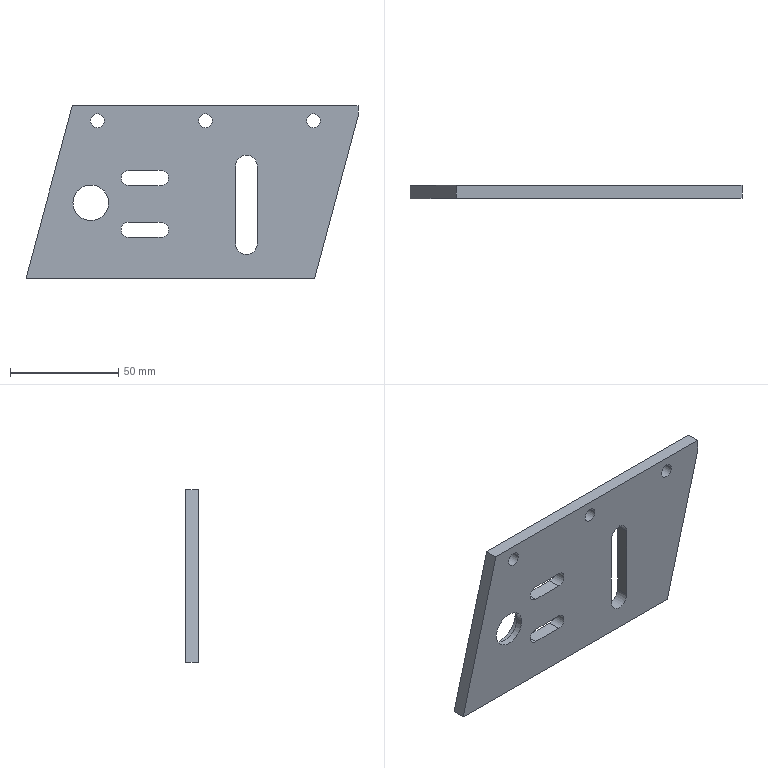Part | SolidWorks | features BaseBody 1 | 1 solid | 32 faces | box 153.66 x 6 x 80 mm | volume 57575 mm3 | cylinder 18 | plane 14 | commonest cylinder face diameters 6.4 x6 7 x6 10 x2 16.5 x2 20 x2
STEP:
#1=CARTESIAN_POINT('',(-37.5,3.,-10.));
#2=VERTEX_POINT('',#1);
#3=CARTESIAN_POINT('',(-37.5,6.,-10.));
#4=VERTEX_POINT('',#3);
#5=CARTESIAN_POINT('',(-37.5,3.,-10.));
#6=DIRECTION('',(0.,1.,0.));
#7=VECTOR('',#6,1000.);
#8=LINE('',#5,#7);
#9=EDGE_CURVE('',#2,#4,#8,.T.);
#10=ORIENTED_EDGE('',*,*,#9,.F.);
#11=CARTESIAN_POINT('',(-57.5,3.,-10.));
#12=VERTEX_POINT('',#11);
#13=CARTESIAN_POINT('',(-47.5,3.,-10.));
#14=DIRECTION('',(0.,1.,0.));
#15=DIRECTION('',(-1.,0.,0.));
#16=AXIS2_PLACEMENT_3D('',#13,#14,#15);
#17=CIRCLE('',#16,10.);
#18=EDGE_CURVE('',#12,#2,#17,.T.);
#19=ORIENTED_EDGE('',*,*,#18,.F.);
#20=CARTESIAN_POINT('',(-57.5,6.,-10.));
#21=VERTEX_POINT('',#20);
#22=CARTESIAN_POINT('',(-57.5,3.,-10.));
#23=DIRECTION('',(0.,1.,0.));
#24=VECTOR('',#23,1000.);
#25=LINE('',#22,#24);
#26=EDGE_CURVE('',#12,#21,#25,.T.);
#27=ORIENTED_EDGE('',*,*,#26,.T.);
#28=CARTESIAN_POINT('',(-47.5,6.,-10.));
#29=DIRECTION('',(0.,-1.,0.));
#30=DIRECTION('',(-1.,0.,0.));
#31=AXIS2_PLACEMENT_3D('',#28,#29,#30);
#32=CIRCLE('',#31,10.);
#33=EDGE_CURVE('',#4,#21,#32,.T.);
#34=ORIENTED_EDGE('',*,*,#33,.F.);
#35=EDGE_LOOP('',(#10,#19,#27,#34));
#36=FACE_OUTER_BOUND('',#35,.T.);
#37=CARTESIAN_POINT('',(-47.5,3.,-10.));
#38=DIRECTION('',(0.,1.,0.));
#39=DIRECTION('',(-1.,0.,0.));
#40=AXIS2_PLACEMENT_3D('',#37,#38,#39);
#41=CYLINDRICAL_SURFACE('',#40,10.);
#42=ADVANCED_FACE('',(#36),#41,.F.);
#43=CARTESIAN_POINT('',(-39.25,3.,-10.));
#44=VERTEX_POINT('',#43);
#45=CARTESIAN_POINT('',(-55.75,3.,-10.));
#46=VERTEX_POINT('',#45);
#47=CARTESIAN_POINT('',(-47.5,3.,-10.));
#48=DIRECTION('',(0.,-1.,0.));
#49=DIRECTION('',(1.,0.,0.));
#50=AXIS2_PLACEMENT_3D('',#47,#48,#49);
#51=CIRCLE('',#50,8.25);
#52=EDGE_CURVE('',#44,#46,#51,.T.);
#53=ORIENTED_EDGE('',*,*,#52,.T.);
#54=CARTESIAN_POINT('',(-47.5,3.,-10.));
#55=DIRECTION('',(0.,-1.,0.));
#56=DIRECTION('',(1.,0.,0.));
#57=AXIS2_PLACEMENT_3D('',#54,#55,#56);
#58=CIRCLE('',#57,8.25);
#59=EDGE_CURVE('',#46,#44,#58,.T.);
#60=ORIENTED_EDGE('',*,*,#59,.T.);
#61=EDGE_LOOP('',(#53,#60));
#62=FACE_BOUND('',#61,.T.);
#63=ORIENTED_EDGE('',*,*,#18,.T.);
#64=CARTESIAN_POINT('',(-47.5,3.,-10.));
#65=DIRECTION('',(0.,1.,0.));
#66=DIRECTION('',(-1.,0.,0.));
#67=AXIS2_PLACEMENT_3D('',#64,#65,#66);
#68=CIRCLE('',#67,10.);
#69=EDGE_CURVE('',#2,#12,#68,.T.);
#70=ORIENTED_EDGE('',*,*,#69,.T.);
#71=EDGE_LOOP('',(#63,#70));
#72=FACE_OUTER_BOUND('',#71,.T.);
#73=CARTESIAN_POINT('',(-47.5,3.,-10.));
#74=DIRECTION('',(0.,1.,0.));
#75=DIRECTION('',(1.,0.,0.));
#76=AXIS2_PLACEMENT_3D('',#73,#74,#75);
#77=PLANE('',#76);
#78=ADVANCED_FACE('',(#62,#72),#77,.T.);
#79=CARTESIAN_POINT('',(-41.3,6.,28.));
#80=VERTEX_POINT('',#79);
#81=CARTESIAN_POINT('',(-47.7,6.,28.));
#82=VERTEX_POINT('',#81);
#83=CARTESIAN_POINT('',(-44.5,6.,28.));
#84=DIRECTION('',(0.,-1.,0.));
#85=DIRECTION('',(1.,0.,0.));
#86=AXIS2_PLACEMENT_3D('',#83,#84,#85);
#87=CIRCLE('',#86,3.2);
#88=EDGE_CURVE('',#80,#82,#87,.T.);
#89=ORIENTED_EDGE('',*,*,#88,.T.);
#90=CARTESIAN_POINT('',(-44.5,6.,28.));
#91=DIRECTION('',(0.,-1.,0.));
#92=DIRECTION('',(1.,0.,0.));
#93=AXIS2_PLACEMENT_3D('',#90,#91,#92);
#94=CIRCLE('',#93,3.2);
#95=EDGE_CURVE('',#82,#80,#94,.T.);
#96=ORIENTED_EDGE('',*,*,#95,.T.);
#97=EDGE_LOOP('',(#89,#96));
#98=FACE_BOUND('',#97,.T.);
#99=CARTESIAN_POINT('',(8.7,6.,28.));
#100=VERTEX_POINT('',#99);
#101=CARTESIAN_POINT('',(2.3,6.,28.));
#102=VERTEX_POINT('',#101);
#103=CARTESIAN_POINT('',(5.5,6.,28.));
#104=DIRECTION('',(0.,-1.,0.));
#105=DIRECTION('',(1.,0.,0.));
#106=AXIS2_PLACEMENT_3D('',#103,#104,#105);
#107=CIRCLE('',#106,3.2);
#108=EDGE_CURVE('',#100,#102,#107,.T.);
#109=ORIENTED_EDGE('',*,*,#108,.T.);
#110=CARTESIAN_POINT('',(5.5,6.,28.));
#111=DIRECTION('',(0.,-1.,0.));
#112=DIRECTION('',(1.,0.,0.));
#113=AXIS2_PLACEMENT_3D('',#110,#111,#112);
#114=CIRCLE('',#113,3.2);
#115=EDGE_CURVE('',#102,#100,#114,.T.);
#116=ORIENTED_EDGE('',*,*,#115,.T.);
#117=EDGE_LOOP('',(#109,#116));
#118=FACE_BOUND('',#117,.T.);
#119=CARTESIAN_POINT('',(58.7,6.,28.));
#120=VERTEX_POINT('',#119);
#121=CARTESIAN_POINT('',(52.3,6.,28.));
#122=VERTEX_POINT('',#121);
#123=CARTESIAN_POINT('',(55.5,6.,28.));
#124=DIRECTION('',(0.,-1.,0.));
#125=DIRECTION('',(1.,0.,0.));
#126=AXIS2_PLACEMENT_3D('',#123,#124,#125);
#127=CIRCLE('',#126,3.2);
#128=EDGE_CURVE('',#120,#122,#127,.T.);
#129=ORIENTED_EDGE('',*,*,#128,.T.);
#130=CARTESIAN_POINT('',(55.5,6.,28.));
#131=DIRECTION('',(0.,-1.,0.));
#132=DIRECTION('',(1.,0.,0.));
#133=AXIS2_PLACEMENT_3D('',#130,#131,#132);
#134=CIRCLE('',#133,3.2);
#135=EDGE_CURVE('',#122,#120,#134,.T.);
#136=ORIENTED_EDGE('',*,*,#135,.T.);
#137=EDGE_LOOP('',(#129,#136));
#138=FACE_BOUND('',#137,.T.);
#139=CARTESIAN_POINT('',(19.5,6.,-29.));
#140=VERTEX_POINT('',#139);
#141=CARTESIAN_POINT('',(29.5,6.,-29.));
#142=VERTEX_POINT('',#141);
#143=CARTESIAN_POINT('',(24.5,6.,-29.));
#144=DIRECTION('',(0.,-1.,0.));
#145=DIRECTION('',(-1.,0.,0.));
#146=AXIS2_PLACEMENT_3D('',#143,#144,#145);
#147=CIRCLE('',#146,5.);
#148=EDGE_CURVE('',#140,#142,#147,.T.);
#149=ORIENTED_EDGE('',*,*,#148,.T.);
#150=CARTESIAN_POINT('',(29.5,6.,7.));
#151=VERTEX_POINT('',#150);
#152=CARTESIAN_POINT('',(29.5,6.,-29.));
#153=DIRECTION('',(0.,0.,1.));
#154=VECTOR('',#153,1000.);
#155=LINE('',#152,#154);
#156=EDGE_CURVE('',#142,#151,#155,.T.);
#157=ORIENTED_EDGE('',*,*,#156,.T.);
#158=CARTESIAN_POINT('',(19.5,6.,7.));
#159=VERTEX_POINT('',#158);
#160=CARTESIAN_POINT('',(24.5,6.,7.));
#161=DIRECTION('',(0.,-1.,0.));
#162=DIRECTION('',(-1.,0.,0.));
#163=AXIS2_PLACEMENT_3D('',#160,#161,#162);
#164=CIRCLE('',#163,5.);
#165=EDGE_CURVE('',#151,#159,#164,.T.);
#166=ORIENTED_EDGE('',*,*,#165,.T.);
#167=CARTESIAN_POINT('',(19.5,6.,-29.));
#168=DIRECTION('',(0.,0.,-1.));
#169=VECTOR('',#168,1000.);
#170=LINE('',#167,#169);
#171=EDGE_CURVE('',#159,#140,#170,.T.);
#172=ORIENTED_EDGE('',*,*,#171,.T.);
#173=EDGE_LOOP('',(#149,#157,#166,#172));
#174=FACE_BOUND('',#173,.T.);
#175=CARTESIAN_POINT('',(-47.5,6.,-10.));
#176=DIRECTION('',(0.,-1.,0.));
#177=DIRECTION('',(-1.,0.,0.));
#178=AXIS2_PLACEMENT_3D('',#175,#176,#177);
#179=CIRCLE('',#178,10.);
#180=EDGE_CURVE('',#21,#4,#179,.T.);
#181=ORIENTED_EDGE('',*,*,#180,.T.);
#182=ORIENTED_EDGE('',*,*,#33,.T.);
#183=EDGE_LOOP('',(#181,#182));
#184=FACE_BOUND('',#183,.T.);
#185=CARTESIAN_POINT('',(-30.,6.,-19.));
#186=VERTEX_POINT('',#185);
#187=CARTESIAN_POINT('',(-33.5,6.,-22.5));
#188=VERTEX_POINT('',#187);
#189=CARTESIAN_POINT('',(-30.,6.,-22.5));
#190=DIRECTION('',(0.,-1.,0.));
#191=DIRECTION('',(-1.,0.,0.));
#192=AXIS2_PLACEMENT_3D('',#189,#190,#191);
#193=CIRCLE('',#192,3.5);
#194=EDGE_CURVE('',#186,#188,#193,.T.);
#195=ORIENTED_EDGE('',*,*,#194,.T.);
#196=CARTESIAN_POINT('',(-30.,6.,-26.));
#197=VERTEX_POINT('',#196);
#198=CARTESIAN_POINT('',(-30.,6.,-22.5));
#199=DIRECTION('',(0.,-1.,0.));
#200=DIRECTION('',(-1.,0.,0.));
#201=AXIS2_PLACEMENT_3D('',#198,#199,#200);
#202=CIRCLE('',#201,3.5);
#203=EDGE_CURVE('',#188,#197,#202,.T.);
#204=ORIENTED_EDGE('',*,*,#203,.T.);
#205=CARTESIAN_POINT('',(-15.,6.,-26.));
#206=VERTEX_POINT('',#205);
#207=CARTESIAN_POINT('',(-30.,6.,-26.));
#208=DIRECTION('',(1.,0.,0.));
#209=VECTOR('',#208,1000.);
#210=LINE('',#207,#209);
#211=EDGE_CURVE('',#197,#206,#210,.T.);
#212=ORIENTED_EDGE('',*,*,#211,.T.);
#213=CARTESIAN_POINT('',(-15.,6.,-19.));
#214=VERTEX_POINT('',#213);
#215=CARTESIAN_POINT('',(-15.,6.,-22.5));
#216=DIRECTION('',(0.,-1.,0.));
#217=DIRECTION('',(-1.,0.,0.));
#218=AXIS2_PLACEMENT_3D('',#215,#216,#217);
#219=CIRCLE('',#218,3.5);
#220=EDGE_CURVE('',#206,#214,#219,.T.);
#221=ORIENTED_EDGE('',*,*,#220,.T.);
#222=CARTESIAN_POINT('',(-30.,6.,-19.));
#223=DIRECTION('',(-1.,0.,0.));
#224=VECTOR('',#223,1000.);
#225=LINE('',#222,#224);
#226=EDGE_CURVE('',#214,#186,#225,.T.);
#227=ORIENTED_EDGE('',*,*,#226,.T.);
#228=EDGE_LOOP('',(#195,#204,#212,#221,#227));
#229=FACE_BOUND('',#228,.T.);
#230=CARTESIAN_POINT('',(-30.,6.,5.));
#231=VERTEX_POINT('',#230);
#232=CARTESIAN_POINT('',(-33.5,6.,1.5));
#233=VERTEX_POINT('',#232);
#234=CARTESIAN_POINT('',(-30.,6.,1.5));
#235=DIRECTION('',(0.,-1.,0.));
#236=DIRECTION('',(-1.,0.,0.));
#237=AXIS2_PLACEMENT_3D('',#234,#235,#236);
#238=CIRCLE('',#237,3.5);
#239=EDGE_CURVE('',#231,#233,#238,.T.);
#240=ORIENTED_EDGE('',*,*,#239,.T.);
#241=CARTESIAN_POINT('',(-30.,6.,-2.));
#242=VERTEX_POINT('',#241);
#243=CARTESIAN_POINT('',(-30.,6.,1.5));
#244=DIRECTION('',(0.,-1.,0.));
#245=DIRECTION('',(-1.,0.,0.));
#246=AXIS2_PLACEMENT_3D('',#243,#244,#245);
#247=CIRCLE('',#246,3.5);
#248=EDGE_CURVE('',#233,#242,#247,.T.);
#249=ORIENTED_EDGE('',*,*,#248,.T.);
#250=CARTESIAN_POINT('',(-15.,6.,-2.));
#251=VERTEX_POINT('',#250);
#252=CARTESIAN_POINT('',(-30.,6.,-2.));
#253=DIRECTION('',(1.,0.,0.));
#254=VECTOR('',#253,1000.);
#255=LINE('',#252,#254);
#256=EDGE_CURVE('',#242,#251,#255,.T.);
#257=ORIENTED_EDGE('',*,*,#256,.T.);
#258=CARTESIAN_POINT('',(-15.,6.,5.));
#259=VERTEX_POINT('',#258);
#260=CARTESIAN_POINT('',(-15.,6.,1.5));
#261=DIRECTION('',(0.,-1.,0.));
#262=DIRECTION('',(-1.,0.,0.));
#263=AXIS2_PLACEMENT_3D('',#260,#261,#262);
#264=CIRCLE('',#263,3.5);
#265=EDGE_CURVE('',#251,#259,#264,.T.);
#266=ORIENTED_EDGE('',*,*,#265,.T.);
#267=CARTESIAN_POINT('',(-30.,6.,5.));
#268=DIRECTION('',(-1.,0.,0.));
#269=VECTOR('',#268,1000.);
#270=LINE('',#267,#269);
#271=EDGE_CURVE('',#259,#231,#270,.T.);
#272=ORIENTED_EDGE('',*,*,#271,.T.);
#273=EDGE_LOOP('',(#240,#249,#257,#266,#272));
#274=FACE_BOUND('',#273,.T.);
#275=CARTESIAN_POINT('',(76.16,6.,30.));
#276=VERTEX_POINT('',#275);
#277=CARTESIAN_POINT('',(56.064,6.,-45.));
#278=VERTEX_POINT('',#277);
#279=CARTESIAN_POINT('',(77.5,6.,35.));
#280=DIRECTION('',(-0.2588,0.,-0.9659));
#281=VECTOR('',#280,1000.);
#282=LINE('',#279,#281);
#283=EDGE_CURVE('',#276,#278,#282,.T.);
#284=ORIENTED_EDGE('',*,*,#283,.T.);
#285=CARTESIAN_POINT('',(-77.5,6.,-45.));
#286=VERTEX_POINT('',#285);
#287=CARTESIAN_POINT('',(-77.5,6.,-45.));
#288=DIRECTION('',(-1.,0.,0.));
#289=VECTOR('',#288,1000.);
#290=LINE('',#287,#289);
#291=EDGE_CURVE('',#278,#286,#290,.T.);
#292=ORIENTED_EDGE('',*,*,#291,.T.);
#293=CARTESIAN_POINT('',(-56.064,6.,35.));
#294=VERTEX_POINT('',#293);
#295=CARTESIAN_POINT('',(-77.5,6.,-45.));
#296=DIRECTION('',(0.2588,0.,0.9659));
#297=VECTOR('',#296,1000.);
#298=LINE('',#295,#297);
#299=EDGE_CURVE('',#286,#294,#298,.T.);
#300=ORIENTED_EDGE('',*,*,#299,.T.);
#301=CARTESIAN_POINT('',(76.16,6.,35.));
#302=VERTEX_POINT('',#301);
#303=CARTESIAN_POINT('',(-77.5,6.,35.));
#304=DIRECTION('',(1.,0.,0.));
#305=VECTOR('',#304,1000.);
#306=LINE('',#303,#305);
#307=EDGE_CURVE('',#294,#302,#306,.T.);
#308=ORIENTED_EDGE('',*,*,#307,.T.);
#309=CARTESIAN_POINT('',(76.16,6.,35.));
#310=DIRECTION('',(0.,0.,-1.));
#311=VECTOR('',#310,1000.);
#312=LINE('',#309,#311);
#313=EDGE_CURVE('',#302,#276,#312,.T.);
#314=ORIENTED_EDGE('',*,*,#313,.T.);
#315=EDGE_LOOP('',(#284,#292,#300,#308,#314));
#316=FACE_OUTER_BOUND('',#315,.T.);
#317=CARTESIAN_POINT('',(0.,6.,0.));
#318=DIRECTION('',(0.,1.,0.));
#319=DIRECTION('',(1.,0.,0.));
#320=AXIS2_PLACEMENT_3D('',#317,#318,#319);
#321=PLANE('',#320);
#322=ADVANCED_FACE('',(#98,#118,#138,#174,#184,#229,#274,#316),#321,.T.);
#323=CARTESIAN_POINT('',(76.16,0.,30.));
#324=VERTEX_POINT('',#323);
#325=CARTESIAN_POINT('',(56.064,0.,-45.));
#326=VERTEX_POINT('',#325);
#327=CARTESIAN_POINT('',(76.16,0.,30.));
#328=DIRECTION('',(-0.2588,0.,-0.9659));
#329=VECTOR('',#328,1000.);
#330=LINE('',#327,#329);
#331=EDGE_CURVE('',#324,#326,#330,.T.);
#332=ORIENTED_EDGE('',*,*,#331,.T.);
#333=CARTESIAN_POINT('',(56.064,6.,-45.));
#334=DIRECTION('',(0.,1.,0.));
#335=VECTOR('',#334,1000.);
#336=LINE('',#333,#335);
#337=EDGE_CURVE('',#326,#278,#336,.T.);
#338=ORIENTED_EDGE('',*,*,#337,.T.);
#339=ORIENTED_EDGE('',*,*,#283,.F.);
#340=CARTESIAN_POINT('',(76.16,6.,30.));
#341=DIRECTION('',(0.,-1.,0.));
#342=VECTOR('',#341,1000.);
#343=LINE('',#340,#342);
#344=EDGE_CURVE('',#276,#324,#343,.T.);
#345=ORIENTED_EDGE('',*,*,#344,.T.);
#346=EDGE_LOOP('',(#332,#338,#339,#345));
#347=FACE_OUTER_BOUND('',#346,.T.);
#348=CARTESIAN_POINT('',(77.5,0.,35.));
#349=DIRECTION('',(-0.9659,0.,0.2588));
#350=DIRECTION('',(0.,1.,0.));
#351=AXIS2_PLACEMENT_3D('',#348,#349,#350);
#352=PLANE('',#351);
#353=ADVANCED_FACE('',(#347),#352,.F.);
#354=CARTESIAN_POINT('',(-77.5,0.,-45.));
#355=VERTEX_POINT('',#354);
#356=CARTESIAN_POINT('',(0.,0.,-45.));
#357=DIRECTION('',(-1.,0.,0.));
#358=VECTOR('',#357,1000.);
#359=LINE('',#356,#358);
#360=EDGE_CURVE('',#326,#355,#359,.T.);
#361=ORIENTED_EDGE('',*,*,#360,.T.);
#362=CARTESIAN_POINT('',(-77.5,0.,-45.));
#363=DIRECTION('',(0.,1.,0.));
#364=VECTOR('',#363,1000.);
#365=LINE('',#362,#364);
#366=EDGE_CURVE('',#355,#286,#365,.T.);
#367=ORIENTED_EDGE('',*,*,#366,.T.);
#368=ORIENTED_EDGE('',*,*,#291,.F.);
#369=ORIENTED_EDGE('',*,*,#337,.F.);
#370=EDGE_LOOP('',(#361,#367,#368,#369));
#371=FACE_OUTER_BOUND('',#370,.T.);
#372=CARTESIAN_POINT('',(-77.5,6.,-45.));
#373=DIRECTION('',(0.,0.,1.));
#374=DIRECTION('',(0.,-1.,0.));
#375=AXIS2_PLACEMENT_3D('',#372,#373,#374);
#376=PLANE('',#375);
#377=ADVANCED_FACE('',(#371),#376,.F.);
#378=ORIENTED_EDGE('',*,*,#299,.F.);
#379=ORIENTED_EDGE('',*,*,#366,.F.);
#380=CARTESIAN_POINT('',(-56.064,0.,35.));
#381=VERTEX_POINT('',#380);
#382=CARTESIAN_POINT('',(-77.5,0.,-45.));
#383=DIRECTION('',(0.2588,0.,0.9659));
#384=VECTOR('',#383,1000.);
#385=LINE('',#382,#384);
#386=EDGE_CURVE('',#355,#381,#385,.T.);
#387=ORIENTED_EDGE('',*,*,#386,.T.);
#388=CARTESIAN_POINT('',(-56.064,6.,35.));
#389=DIRECTION('',(0.,1.,0.));
#390=VECTOR('',#389,1000.);
#391=LINE('',#388,#390);
#392=EDGE_CURVE('',#381,#294,#391,.T.);
#393=ORIENTED_EDGE('',*,*,#392,.T.);
#394=EDGE_LOOP('',(#378,#379,#387,#393));
#395=FACE_OUTER_BOUND('',#394,.T.);
#396=CARTESIAN_POINT('',(-77.5,0.,-45.));
#397=DIRECTION('',(0.9659,0.,-0.2588));
#398=DIRECTION('',(0.,-1.,0.));
#399=AXIS2_PLACEMENT_3D('',#396,#397,#398);
#400=PLANE('',#399);
#401=ADVANCED_FACE('',(#395),#400,.F.);
#402=ORIENTED_EDGE('',*,*,#307,.F.);
#403=ORIENTED_EDGE('',*,*,#392,.F.);
#404=CARTESIAN_POINT('',(76.16,0.,35.));
#405=VERTEX_POINT('',#404);
#406=CARTESIAN_POINT('',(0.,0.,35.));
#407=DIRECTION('',(1.,0.,0.));
#408=VECTOR('',#407,1000.);
#409=LINE('',#406,#408);
#410=EDGE_CURVE('',#381,#405,#409,.T.);
#411=ORIENTED_EDGE('',*,*,#410,.T.);
#412=CARTESIAN_POINT('',(76.16,6.,35.));
#413=DIRECTION('',(0.,1.,0.));
#414=VECTOR('',#413,1000.);
#415=LINE('',#412,#414);
#416=EDGE_CURVE('',#405,#302,#415,.T.);
#417=ORIENTED_EDGE('',*,*,#416,.T.);
#418=EDGE_LOOP('',(#402,#403,#411,#417));
#419=FACE_OUTER_BOUND('',#418,.T.);
#420=CARTESIAN_POINT('',(-77.5,6.,35.));
#421=DIRECTION('',(0.,0.,-1.));
#422=DIRECTION('',(-1.,0.,0.));
#423=AXIS2_PLACEMENT_3D('',#420,#421,#422);
#424=PLANE('',#423);
#425=ADVANCED_FACE('',(#419),#424,.F.);
#426=ORIENTED_EDGE('',*,*,#313,.F.);
#427=ORIENTED_EDGE('',*,*,#416,.F.);
#428=CARTESIAN_POINT('',(76.16,0.,0.));
#429=DIRECTION('',(0.,0.,-1.));
#430=VECTOR('',#429,1000.);
#431=LINE('',#428,#430);
#432=EDGE_CURVE('',#405,#324,#431,.T.);
#433=ORIENTED_EDGE('',*,*,#432,.T.);
#434=ORIENTED_EDGE('',*,*,#344,.F.);
#435=EDGE_LOOP('',(#426,#427,#433,#434));
#436=FACE_OUTER_BOUND('',#435,.T.);
#437=CARTESIAN_POINT('',(76.16,6.,35.));
#438=DIRECTION('',(-1.,0.,0.));
#439=DIRECTION('',(0.,0.,1.));
#440=AXIS2_PLACEMENT_3D('',#437,#438,#439);
#441=PLANE('',#440);
#442=ADVANCED_FACE('',(#436),#441,.F.);
#443=CARTESIAN_POINT('',(-47.7,0.,28.));
#444=VERTEX_POINT('',#443);
#445=CARTESIAN_POINT('',(-47.7,0.,28.));
#446=DIRECTION('',(0.,-1.,0.));
#447=VECTOR('',#446,1000.);
#448=LINE('',#445,#447);
#449=EDGE_CURVE('',#82,#444,#448,.T.);
#450=ORIENTED_EDGE('',*,*,#449,.F.);
#451=ORIENTED_EDGE('',*,*,#88,.F.);
#452=CARTESIAN_POINT('',(-41.3,0.,28.));
#453=VERTEX_POINT('',#452);
#454=CARTESIAN_POINT('',(-41.3,0.,28.));
#455=DIRECTION('',(0.,-1.,0.));
#456=VECTOR('',#455,1000.);
#457=LINE('',#454,#456);
#458=EDGE_CURVE('',#80,#453,#457,.T.);
#459=ORIENTED_EDGE('',*,*,#458,.T.);
#460=CARTESIAN_POINT('',(-44.5,0.,28.));
#461=DIRECTION('',(0.,-1.,0.));
#462=DIRECTION('',(1.,0.,0.));
#463=AXIS2_PLACEMENT_3D('',#460,#461,#462);
#464=CIRCLE('',#463,3.2);
#465=EDGE_CURVE('',#453,#444,#464,.T.);
#466=ORIENTED_EDGE('',*,*,#465,.T.);
#467=EDGE_LOOP('',(#450,#451,#459,#466));
#468=FACE_OUTER_BOUND('',#467,.T.);
#469=CARTESIAN_POINT('',(-44.5,0.,28.));
#470=DIRECTION('',(0.,-1.,0.));
#471=DIRECTION('',(1.,0.,0.));
#472=AXIS2_PLACEMENT_3D('',#469,#470,#471);
#473=CYLINDRICAL_SURFACE('',#472,3.2);
#474=ADVANCED_FACE('',(#468),#473,.F.);
#475=CARTESIAN_POINT('',(2.3,0.,28.));
#476=VERTEX_POINT('',#475);
#477=CARTESIAN_POINT('',(2.3,0.,28.));
#478=DIRECTION('',(0.,-1.,0.));
#479=VECTOR('',#478,1000.);
#480=LINE('',#477,#479);
#481=EDGE_CURVE('',#102,#476,#480,.T.);
#482=ORIENTED_EDGE('',*,*,#481,.F.);
#483=ORIENTED_EDGE('',*,*,#108,.F.);
#484=CARTESIAN_POINT('',(8.7,0.,28.));
#485=VERTEX_POINT('',#484);
#486=CARTESIAN_POINT('',(8.7,0.,28.));
#487=DIRECTION('',(0.,-1.,0.));
#488=VECTOR('',#487,1000.);
#489=LINE('',#486,#488);
#490=EDGE_CURVE('',#100,#485,#489,.T.);
#491=ORIENTED_EDGE('',*,*,#490,.T.);
#492=CARTESIAN_POINT('',(5.5,0.,28.));
#493=DIRECTION('',(0.,-1.,0.));
#494=DIRECTION('',(1.,0.,0.));
#495=AXIS2_PLACEMENT_3D('',#492,#493,#494);
#496=CIRCLE('',#495,3.2);
#497=EDGE_CURVE('',#485,#476,#496,.T.);
#498=ORIENTED_EDGE('',*,*,#497,.T.);
#499=EDGE_LOOP('',(#482,#483,#491,#498));
#500=FACE_OUTER_BOUND('',#499,.T.);
#501=CARTESIAN_POINT('',(5.5,0.,28.));
#502=DIRECTION('',(0.,-1.,0.));
#503=DIRECTION('',(1.,0.,0.));
#504=AXIS2_PLACEMENT_3D('',#501,#502,#503);
#505=CYLINDRICAL_SURFACE('',#504,3.2);
#506=ADVANCED_FACE('',(#500),#505,.F.);
#507=CARTESIAN_POINT('',(52.3,0.,28.));
#508=VERTEX_POINT('',#507);
#509=CARTESIAN_POINT('',(52.3,0.,28.));
#510=DIRECTION('',(0.,-1.,0.));
#511=VECTOR('',#510,1000.);
#512=LINE('',#509,#511);
#513=EDGE_CURVE('',#122,#508,#512,.T.);
#514=ORIENTED_EDGE('',*,*,#513,.F.);
#515=ORIENTED_EDGE('',*,*,#128,.F.);
#516=CARTESIAN_POINT('',(58.7,0.,28.));
#517=VERTEX_POINT('',#516);
#518=CARTESIAN_POINT('',(58.7,0.,28.));
#519=DIRECTION('',(0.,-1.,0.));
#520=VECTOR('',#519,1000.);
#521=LINE('',#518,#520);
#522=EDGE_CURVE('',#120,#517,#521,.T.);
#523=ORIENTED_EDGE('',*,*,#522,.T.);
#524=CARTESIAN_POINT('',(55.5,0.,28.));
#525=DIRECTION('',(0.,-1.,0.));
#526=DIRECTION('',(1.,0.,0.));
#527=AXIS2_PLACEMENT_3D('',#524,#525,#526);
#528=CIRCLE('',#527,3.2);
#529=EDGE_CURVE('',#517,#508,#528,.T.);
#530=ORIENTED_EDGE('',*,*,#529,.T.);
#531=EDGE_LOOP('',(#514,#515,#523,#530));
#532=FACE_OUTER_BOUND('',#531,.T.);
#533=CARTESIAN_POINT('',(55.5,0.,28.));
#534=DIRECTION('',(0.,-1.,0.));
#535=DIRECTION('',(1.,0.,0.));
#536=AXIS2_PLACEMENT_3D('',#533,#534,#535);
#537=CYLINDRICAL_SURFACE('',#536,3.2);
#538=ADVANCED_FACE('',(#532),#537,.F.);
#539=CARTESIAN_POINT('',(29.5,0.,-29.));
#540=VERTEX_POINT('',#539);
#541=CARTESIAN_POINT('',(29.5,0.,7.));
#542=VERTEX_POINT('',#541);
#543=CARTESIAN_POINT('',(29.5,0.,0.));
#544=DIRECTION('',(0.,0.,1.));
#545=VECTOR('',#544,1000.);
#546=LINE('',#543,#545);
#547=EDGE_CURVE('',#540,#542,#546,.T.);
#548=ORIENTED_EDGE('',*,*,#547,.T.);
#549=CARTESIAN_POINT('',(29.5,0.,7.));
#550=DIRECTION('',(0.,1.,0.));
#551=VECTOR('',#550,1000.);
#552=LINE('',#549,#551);
#553=EDGE_CURVE('',#542,#151,#552,.T.);
#554=ORIENTED_EDGE('',*,*,#553,.T.);
#555=ORIENTED_EDGE('',*,*,#156,.F.);
#556=CARTESIAN_POINT('',(29.5,0.,-29.));
#557=DIRECTION('',(0.,-1.,0.));
#558=VECTOR('',#557,1000.);
#559=LINE('',#556,#558);
#560=EDGE_CURVE('',#142,#540,#559,.T.);
#561=ORIENTED_EDGE('',*,*,#560,.T.);
#562=EDGE_LOOP('',(#548,#554,#555,#561));
#563=FACE_OUTER_BOUND('',#562,.T.);
#564=CARTESIAN_POINT('',(29.5,0.,-29.));
#565=DIRECTION('',(1.,0.,0.));
#566=DIRECTION('',(0.,0.,-1.));
#567=AXIS2_PLACEMENT_3D('',#564,#565,#566);
#568=PLANE('',#567);
#569=ADVANCED_FACE('',(#563),#568,.F.);
#570=CARTESIAN_POINT('',(19.5,0.,7.));
#571=VERTEX_POINT('',#570);
#572=CARTESIAN_POINT('',(24.5,0.,7.));
#573=DIRECTION('',(0.,-1.,0.));
#574=DIRECTION('',(-1.,0.,0.));
#575=AXIS2_PLACEMENT_3D('',#572,#573,#574);
#576=CIRCLE('',#575,5.);
#577=EDGE_CURVE('',#542,#571,#576,.T.);
#578=ORIENTED_EDGE('',*,*,#577,.T.);
#579=CARTESIAN_POINT('',(19.5,0.,7.));
#580=DIRECTION('',(0.,1.,0.));
#581=VECTOR('',#580,1000.);
#582=LINE('',#579,#581);
#583=EDGE_CURVE('',#571,#159,#582,.T.);
#584=ORIENTED_EDGE('',*,*,#583,.T.);
#585=ORIENTED_EDGE('',*,*,#165,.F.);
#586=ORIENTED_EDGE('',*,*,#553,.F.);
#587=EDGE_LOOP('',(#578,#584,#585,#586));
#588=FACE_OUTER_BOUND('',#587,.T.);
#589=CARTESIAN_POINT('',(24.5,0.,7.));
#590=DIRECTION('',(0.,1.,0.));
#591=DIRECTION('',(-1.,0.,0.));
#592=AXIS2_PLACEMENT_3D('',#589,#590,#591);
#593=CYLINDRICAL_SURFACE('',#592,5.);
#594=ADVANCED_FACE('',(#588),#593,.F.);
#595=CARTESIAN_POINT('',(19.5,0.,-29.));
#596=VERTEX_POINT('',#595);
#597=CARTESIAN_POINT('',(19.5,0.,0.));
#598=DIRECTION('',(0.,0.,-1.));
#599=VECTOR('',#598,1000.);
#600=LINE('',#597,#599);
#601=EDGE_CURVE('',#571,#596,#600,.T.);
#602=ORIENTED_EDGE('',*,*,#601,.T.);
#603=CARTESIAN_POINT('',(19.5,0.,-29.));
#604=DIRECTION('',(0.,1.,0.));
#605=VECTOR('',#604,1000.);
#606=LINE('',#603,#605);
#607=EDGE_CURVE('',#596,#140,#606,.T.);
#608=ORIENTED_EDGE('',*,*,#607,.T.);
#609=ORIENTED_EDGE('',*,*,#171,.F.);
#610=ORIENTED_EDGE('',*,*,#583,.F.);
#611=EDGE_LOOP('',(#602,#608,#609,#610));
#612=FACE_OUTER_BOUND('',#611,.T.);
#613=CARTESIAN_POINT('',(19.5,0.,-29.));
#614=DIRECTION('',(-1.,0.,0.));
#615=DIRECTION('',(0.,1.,0.));
#616=AXIS2_PLACEMENT_3D('',#613,#614,#615);
#617=PLANE('',#616);
#618=ADVANCED_FACE('',(#612),#617,.F.);
#619=CARTESIAN_POINT('',(24.5,0.,-29.));
#620=DIRECTION('',(0.,-1.,0.));
#621=DIRECTION('',(-1.,0.,0.));
#622=AXIS2_PLACEMENT_3D('',#619,#620,#621);
#623=CIRCLE('',#622,5.);
#624=EDGE_CURVE('',#596,#540,#623,.T.);
#625=ORIENTED_EDGE('',*,*,#624,.T.);
#626=ORIENTED_EDGE('',*,*,#560,.F.);
#627=ORIENTED_EDGE('',*,*,#148,.F.);
#628=ORIENTED_EDGE('',*,*,#607,.F.);
#629=EDGE_LOOP('',(#625,#626,#627,#628));
#630=FACE_OUTER_BOUND('',#629,.T.);
#631=CARTESIAN_POINT('',(24.5,0.,-29.));
#632=DIRECTION('',(0.,1.,0.));
#633=DIRECTION('',(-1.,0.,0.));
#634=AXIS2_PLACEMENT_3D('',#631,#632,#633);
#635=CYLINDRICAL_SURFACE('',#634,5.);
#636=ADVANCED_FACE('',(#630),#635,.F.);
#637=CARTESIAN_POINT('',(-55.75,0.,-10.));
#638=VERTEX_POINT('',#637);
#639=CARTESIAN_POINT('',(-55.75,0.,-10.));
#640=DIRECTION('',(0.,-1.,0.));
#641=VECTOR('',#640,1000.);
#642=LINE('',#639,#641);
#643=EDGE_CURVE('',#46,#638,#642,.T.);
#644=ORIENTED_EDGE('',*,*,#643,.F.);
#645=ORIENTED_EDGE('',*,*,#52,.F.);
#646=CARTESIAN_POINT('',(-39.25,0.,-10.));
#647=VERTEX_POINT('',#646);
#648=CARTESIAN_POINT('',(-39.25,0.,-10.));
#649=DIRECTION('',(0.,-1.,0.));
#650=VECTOR('',#649,1000.);
#651=LINE('',#648,#650);
#652=EDGE_CURVE('',#44,#647,#651,.T.);
#653=ORIENTED_EDGE('',*,*,#652,.T.);
#654=CARTESIAN_POINT('',(-47.5,0.,-10.));
#655=DIRECTION('',(0.,-1.,0.));
#656=DIRECTION('',(1.,0.,0.));
#657=AXIS2_PLACEMENT_3D('',#654,#655,#656);
#658=CIRCLE('',#657,8.25);
#659=EDGE_CURVE('',#647,#638,#658,.T.);
#660=ORIENTED_EDGE('',*,*,#659,.T.);
#661=EDGE_LOOP('',(#644,#645,#653,#660));
#662=FACE_OUTER_BOUND('',#661,.T.);
#663=CARTESIAN_POINT('',(-47.5,0.,-10.));
#664=DIRECTION('',(0.,-1.,0.));
#665=DIRECTION('',(1.,0.,0.));
#666=AXIS2_PLACEMENT_3D('',#663,#664,#665);
#667=CYLINDRICAL_SURFACE('',#666,8.25);
#668=ADVANCED_FACE('',(#662),#667,.F.);
#669=CARTESIAN_POINT('',(-30.,0.,-26.));
#670=VERTEX_POINT('',#669);
#671=CARTESIAN_POINT('',(-15.,0.,-26.));
#672=VERTEX_POINT('',#671);
#673=CARTESIAN_POINT('',(0.,0.,-26.));
#674=DIRECTION('',(1.,0.,0.));
#675=VECTOR('',#674,1000.);
#676=LINE('',#673,#675);
#677=EDGE_CURVE('',#670,#672,#676,.T.);
#678=ORIENTED_EDGE('',*,*,#677,.T.);
#679=CARTESIAN_POINT('',(-15.,0.,-26.));
#680=DIRECTION('',(0.,1.,0.));
#681=VECTOR('',#680,1000.);
#682=LINE('',#679,#681);
#683=EDGE_CURVE('',#672,#206,#682,.T.);
#684=ORIENTED_EDGE('',*,*,#683,.T.);
#685=ORIENTED_EDGE('',*,*,#211,.F.);
#686=CARTESIAN_POINT('',(-30.,0.,-26.));
#687=DIRECTION('',(0.,-1.,0.));
#688=VECTOR('',#687,1000.);
#689=LINE('',#686,#688);
#690=EDGE_CURVE('',#197,#670,#689,.T.);
#691=ORIENTED_EDGE('',*,*,#690,.T.);
#692=EDGE_LOOP('',(#678,#684,#685,#691));
#693=FACE_OUTER_BOUND('',#692,.T.);
#694=CARTESIAN_POINT('',(-30.,0.,-26.));
#695=DIRECTION('',(0.,0.,-1.));
#696=DIRECTION('',(-1.,0.,0.));
#697=AXIS2_PLACEMENT_3D('',#694,#695,#696);
#698=PLANE('',#697);
#699=ADVANCED_FACE('',(#693),#698,.F.);
#700=CARTESIAN_POINT('',(-15.,0.,-19.));
#701=VERTEX_POINT('',#700);
#702=CARTESIAN_POINT('',(-15.,0.,-22.5));
#703=DIRECTION('',(0.,-1.,0.));
#704=DIRECTION('',(-1.,0.,0.));
#705=AXIS2_PLACEMENT_3D('',#702,#703,#704);
#706=CIRCLE('',#705,3.5);
#707=EDGE_CURVE('',#672,#701,#706,.T.);
#708=ORIENTED_EDGE('',*,*,#707,.T.);
#709=CARTESIAN_POINT('',(-15.,0.,-19.));
#710=DIRECTION('',(0.,1.,0.));
#711=VECTOR('',#710,1000.);
#712=LINE('',#709,#711);
#713=EDGE_CURVE('',#701,#214,#712,.T.);
#714=ORIENTED_EDGE('',*,*,#713,.T.);
#715=ORIENTED_EDGE('',*,*,#220,.F.);
#716=ORIENTED_EDGE('',*,*,#683,.F.);
#717=EDGE_LOOP('',(#708,#714,#715,#716));
#718=FACE_OUTER_BOUND('',#717,.T.);
#719=CARTESIAN_POINT('',(-15.,0.,-22.5));
#720=DIRECTION('',(0.,1.,0.));
#721=DIRECTION('',(-1.,0.,0.));
#722=AXIS2_PLACEMENT_3D('',#719,#720,#721);
#723=CYLINDRICAL_SURFACE('',#722,3.5);
#724=ADVANCED_FACE('',(#718),#723,.F.);
#725=CARTESIAN_POINT('',(-30.,0.,-19.));
#726=VERTEX_POINT('',#725);
#727=CARTESIAN_POINT('',(0.,0.,-19.));
#728=DIRECTION('',(-1.,0.,0.));
#729=VECTOR('',#728,1000.);
#730=LINE('',#727,#729);
#731=EDGE_CURVE('',#701,#726,#730,.T.);
#732=ORIENTED_EDGE('',*,*,#731,.T.);
#733=CARTESIAN_POINT('',(-30.,0.,-19.));
#734=DIRECTION('',(0.,1.,0.));
#735=VECTOR('',#734,1000.);
#736=LINE('',#733,#735);
#737=EDGE_CURVE('',#726,#186,#736,.T.);
#738=ORIENTED_EDGE('',*,*,#737,.T.);
#739=ORIENTED_EDGE('',*,*,#226,.F.);
#740=ORIENTED_EDGE('',*,*,#713,.F.);
#741=EDGE_LOOP('',(#732,#738,#739,#740));
#742=FACE_OUTER_BOUND('',#741,.T.);
#743=CARTESIAN_POINT('',(-30.,0.,-19.));
#744=DIRECTION('',(0.,0.,1.));
#745=DIRECTION('',(1.,0.,0.));
#746=AXIS2_PLACEMENT_3D('',#743,#744,#745);
#747=PLANE('',#746);
#748=ADVANCED_FACE('',(#742),#747,.F.);
#749=CARTESIAN_POINT('',(-33.5,0.,-22.5));
#750=VERTEX_POINT('',#749);
#751=CARTESIAN_POINT('',(-33.5,0.,-22.5));
#752=DIRECTION('',(0.,1.,0.));
#753=VECTOR('',#752,1000.);
#754=LINE('',#751,#753);
#755=EDGE_CURVE('',#750,#188,#754,.T.);
#756=ORIENTED_EDGE('',*,*,#755,.F.);
#757=CARTESIAN_POINT('',(-30.,0.,-22.5));
#758=DIRECTION('',(0.,-1.,0.));
#759=DIRECTION('',(-1.,0.,0.));
#760=AXIS2_PLACEMENT_3D('',#757,#758,#759);
#761=CIRCLE('',#760,3.5);
#762=EDGE_CURVE('',#750,#670,#761,.T.);
#763=ORIENTED_EDGE('',*,*,#762,.T.);
#764=ORIENTED_EDGE('',*,*,#690,.F.);
#765=ORIENTED_EDGE('',*,*,#203,.F.);
#766=EDGE_LOOP('',(#756,#763,#764,#765));
#767=FACE_OUTER_BOUND('',#766,.T.);
#768=CARTESIAN_POINT('',(-30.,0.,-22.5));
#769=DIRECTION('',(0.,1.,0.));
#770=DIRECTION('',(-1.,0.,0.));
#771=AXIS2_PLACEMENT_3D('',#768,#769,#770);
#772=CYLINDRICAL_SURFACE('',#771,3.5);
#773=ADVANCED_FACE('',(#767),#772,.F.);
#774=CARTESIAN_POINT('',(-30.,0.,-2.));
#775=VERTEX_POINT('',#774);
#776=CARTESIAN_POINT('',(-15.,0.,-2.));
#777=VERTEX_POINT('',#776);
#778=CARTESIAN_POINT('',(0.,0.,-2.));
#779=DIRECTION('',(1.,0.,0.));
#780=VECTOR('',#779,1000.);
#781=LINE('',#778,#780);
#782=EDGE_CURVE('',#775,#777,#781,.T.);
#783=ORIENTED_EDGE('',*,*,#782,.T.);
#784=CARTESIAN_POINT('',(-15.,0.,-2.));
#785=DIRECTION('',(0.,1.,0.));
#786=VECTOR('',#785,1000.);
#787=LINE('',#784,#786);
#788=EDGE_CURVE('',#777,#251,#787,.T.);
#789=ORIENTED_EDGE('',*,*,#788,.T.);
#790=ORIENTED_EDGE('',*,*,#256,.F.);
#791=CARTESIAN_POINT('',(-30.,0.,-2.));
#792=DIRECTION('',(0.,-1.,0.));
#793=VECTOR('',#792,1000.);
#794=LINE('',#791,#793);
#795=EDGE_CURVE('',#242,#775,#794,.T.);
#796=ORIENTED_EDGE('',*,*,#795,.T.);
#797=EDGE_LOOP('',(#783,#789,#790,#796));
#798=FACE_OUTER_BOUND('',#797,.T.);
#799=CARTESIAN_POINT('',(-30.,0.,-2.));
#800=DIRECTION('',(0.,0.,-1.));
#801=DIRECTION('',(-1.,0.,0.));
#802=AXIS2_PLACEMENT_3D('',#799,#800,#801);
#803=PLANE('',#802);
#804=ADVANCED_FACE('',(#798),#803,.F.);
#805=CARTESIAN_POINT('',(-15.,0.,5.));
#806=VERTEX_POINT('',#805);
#807=CARTESIAN_POINT('',(-15.,0.,1.5));
#808=DIRECTION('',(0.,-1.,0.));
#809=DIRECTION('',(-1.,0.,0.));
#810=AXIS2_PLACEMENT_3D('',#807,#808,#809);
#811=CIRCLE('',#810,3.5);
#812=EDGE_CURVE('',#777,#806,#811,.T.);
#813=ORIENTED_EDGE('',*,*,#812,.T.);
#814=CARTESIAN_POINT('',(-15.,0.,5.));
#815=DIRECTION('',(0.,1.,0.));
#816=VECTOR('',#815,1000.);
#817=LINE('',#814,#816);
#818=EDGE_CURVE('',#806,#259,#817,.T.);
#819=ORIENTED_EDGE('',*,*,#818,.T.);
#820=ORIENTED_EDGE('',*,*,#265,.F.);
#821=ORIENTED_EDGE('',*,*,#788,.F.);
#822=EDGE_LOOP('',(#813,#819,#820,#821));
#823=FACE_OUTER_BOUND('',#822,.T.);
#824=CARTESIAN_POINT('',(-15.,0.,1.5));
#825=DIRECTION('',(0.,1.,0.));
#826=DIRECTION('',(-1.,0.,0.));
#827=AXIS2_PLACEMENT_3D('',#824,#825,#826);
#828=CYLINDRICAL_SURFACE('',#827,3.5);
#829=ADVANCED_FACE('',(#823),#828,.F.);
#830=CARTESIAN_POINT('',(-30.,0.,5.));
#831=VERTEX_POINT('',#830);
#832=CARTESIAN_POINT('',(0.,0.,5.));
#833=DIRECTION('',(-1.,0.,0.));
#834=VECTOR('',#833,1000.);
#835=LINE('',#832,#834);
#836=EDGE_CURVE('',#806,#831,#835,.T.);
#837=ORIENTED_EDGE('',*,*,#836,.T.);
#838=CARTESIAN_POINT('',(-30.,0.,5.));
#839=DIRECTION('',(0.,1.,0.));
#840=VECTOR('',#839,1000.);
#841=LINE('',#838,#840);
#842=EDGE_CURVE('',#831,#231,#841,.T.);
#843=ORIENTED_EDGE('',*,*,#842,.T.);
#844=ORIENTED_EDGE('',*,*,#271,.F.);
#845=ORIENTED_EDGE('',*,*,#818,.F.);
#846=EDGE_LOOP('',(#837,#843,#844,#845));
#847=FACE_OUTER_BOUND('',#846,.T.);
#848=CARTESIAN_POINT('',(-30.,0.,5.));
#849=DIRECTION('',(0.,0.,1.));
#850=DIRECTION('',(1.,0.,0.));
#851=AXIS2_PLACEMENT_3D('',#848,#849,#850);
#852=PLANE('',#851);
#853=ADVANCED_FACE('',(#847),#852,.F.);
#854=CARTESIAN_POINT('',(-33.5,0.,1.5));
#855=VERTEX_POINT('',#854);
#856=CARTESIAN_POINT('',(-33.5,0.,1.5));
#857=DIRECTION('',(0.,1.,0.));
#858=VECTOR('',#857,1000.);
#859=LINE('',#856,#858);
#860=EDGE_CURVE('',#855,#233,#859,.T.);
#861=ORIENTED_EDGE('',*,*,#860,.F.);
#862=CARTESIAN_POINT('',(-30.,0.,1.5));
#863=DIRECTION('',(0.,-1.,0.));
#864=DIRECTION('',(-1.,0.,0.));
#865=AXIS2_PLACEMENT_3D('',#862,#863,#864);
#866=CIRCLE('',#865,3.5);
#867=EDGE_CURVE('',#855,#775,#866,.T.);
#868=ORIENTED_EDGE('',*,*,#867,.T.);
#869=ORIENTED_EDGE('',*,*,#795,.F.);
#870=ORIENTED_EDGE('',*,*,#248,.F.);
#871=EDGE_LOOP('',(#861,#868,#869,#870));
#872=FACE_OUTER_BOUND('',#871,.T.);
#873=CARTESIAN_POINT('',(-30.,0.,1.5));
#874=DIRECTION('',(0.,1.,0.));
#875=DIRECTION('',(-1.,0.,0.));
#876=AXIS2_PLACEMENT_3D('',#873,#874,#875);
#877=CYLINDRICAL_SURFACE('',#876,3.5);
#878=ADVANCED_FACE('',(#872),#877,.F.);
#879=ORIENTED_EDGE('',*,*,#465,.F.);
#880=CARTESIAN_POINT('',(-44.5,0.,28.));
#881=DIRECTION('',(0.,-1.,0.));
#882=DIRECTION('',(1.,0.,0.));
#883=AXIS2_PLACEMENT_3D('',#880,#881,#882);
#884=CIRCLE('',#883,3.2);
#885=EDGE_CURVE('',#444,#453,#884,.T.);
#886=ORIENTED_EDGE('',*,*,#885,.F.);
#887=EDGE_LOOP('',(#879,#886));
#888=FACE_BOUND('',#887,.T.);
#889=ORIENTED_EDGE('',*,*,#497,.F.);
#890=CARTESIAN_POINT('',(5.5,0.,28.));
#891=DIRECTION('',(0.,-1.,0.));
#892=DIRECTION('',(1.,0.,0.));
#893=AXIS2_PLACEMENT_3D('',#890,#891,#892);
#894=CIRCLE('',#893,3.2);
#895=EDGE_CURVE('',#476,#485,#894,.T.);
#896=ORIENTED_EDGE('',*,*,#895,.F.);
#897=EDGE_LOOP('',(#889,#896));
#898=FACE_BOUND('',#897,.T.);
#899=ORIENTED_EDGE('',*,*,#529,.F.);
#900=CARTESIAN_POINT('',(55.5,0.,28.));
#901=DIRECTION('',(0.,-1.,0.));
#902=DIRECTION('',(1.,0.,0.));
#903=AXIS2_PLACEMENT_3D('',#900,#901,#902);
#904=CIRCLE('',#903,3.2);
#905=EDGE_CURVE('',#508,#517,#904,.T.);
#906=ORIENTED_EDGE('',*,*,#905,.F.);
#907=EDGE_LOOP('',(#899,#906));
#908=FACE_BOUND('',#907,.T.);
#909=ORIENTED_EDGE('',*,*,#601,.F.);
#910=ORIENTED_EDGE('',*,*,#577,.F.);
#911=ORIENTED_EDGE('',*,*,#547,.F.);
#912=ORIENTED_EDGE('',*,*,#624,.F.);
#913=EDGE_LOOP('',(#909,#910,#911,#912));
#914=FACE_BOUND('',#913,.T.);
#915=ORIENTED_EDGE('',*,*,#659,.F.);
#916=CARTESIAN_POINT('',(-47.5,0.,-10.));
#917=DIRECTION('',(0.,-1.,0.));
#918=DIRECTION('',(1.,0.,0.));
#919=AXIS2_PLACEMENT_3D('',#916,#917,#918);
#920=CIRCLE('',#919,8.25);
#921=EDGE_CURVE('',#638,#647,#920,.T.);
#922=ORIENTED_EDGE('',*,*,#921,.F.);
#923=EDGE_LOOP('',(#915,#922));
#924=FACE_BOUND('',#923,.T.);
#925=ORIENTED_EDGE('',*,*,#731,.F.);
#926=ORIENTED_EDGE('',*,*,#707,.F.);
#927=ORIENTED_EDGE('',*,*,#677,.F.);
#928=ORIENTED_EDGE('',*,*,#762,.F.);
#929=CARTESIAN_POINT('',(-30.,0.,-22.5));
#930=DIRECTION('',(0.,-1.,0.));
#931=DIRECTION('',(-1.,0.,0.));
#932=AXIS2_PLACEMENT_3D('',#929,#930,#931);
#933=CIRCLE('',#932,3.5);
#934=EDGE_CURVE('',#726,#750,#933,.T.);
#935=ORIENTED_EDGE('',*,*,#934,.F.);
#936=EDGE_LOOP('',(#925,#926,#927,#928,#935));
#937=FACE_BOUND('',#936,.T.);
#938=ORIENTED_EDGE('',*,*,#836,.F.);
#939=ORIENTED_EDGE('',*,*,#812,.F.);
#940=ORIENTED_EDGE('',*,*,#782,.F.);
#941=ORIENTED_EDGE('',*,*,#867,.F.);
#942=CARTESIAN_POINT('',(-30.,0.,1.5));
#943=DIRECTION('',(0.,-1.,0.));
#944=DIRECTION('',(-1.,0.,0.));
#945=AXIS2_PLACEMENT_3D('',#942,#943,#944);
#946=CIRCLE('',#945,3.5);
#947=EDGE_CURVE('',#831,#855,#946,.T.);
#948=ORIENTED_EDGE('',*,*,#947,.F.);
#949=EDGE_LOOP('',(#938,#939,#940,#941,#948));
#950=FACE_BOUND('',#949,.T.);
#951=ORIENTED_EDGE('',*,*,#410,.F.);
#952=ORIENTED_EDGE('',*,*,#386,.F.);
#953=ORIENTED_EDGE('',*,*,#360,.F.);
#954=ORIENTED_EDGE('',*,*,#331,.F.);
#955=ORIENTED_EDGE('',*,*,#432,.F.);
#956=EDGE_LOOP('',(#951,#952,#953,#954,#955));
#957=FACE_OUTER_BOUND('',#956,.T.);
#958=CARTESIAN_POINT('',(0.,0.,0.));
#959=DIRECTION('',(0.,1.,0.));
#960=DIRECTION('',(1.,0.,0.));
#961=AXIS2_PLACEMENT_3D('',#958,#959,#960);
#962=PLANE('',#961);
#963=ADVANCED_FACE('',(#888,#898,#908,#914,#924,#937,#950,#957),#962,.F.);
#964=ORIENTED_EDGE('',*,*,#69,.F.);
#965=ORIENTED_EDGE('',*,*,#9,.T.);
#966=ORIENTED_EDGE('',*,*,#180,.F.);
#967=ORIENTED_EDGE('',*,*,#26,.F.);
#968=EDGE_LOOP('',(#964,#965,#966,#967));
#969=FACE_OUTER_BOUND('',#968,.T.);
#970=CARTESIAN_POINT('',(-47.5,3.,-10.));
#971=DIRECTION('',(0.,1.,0.));
#972=DIRECTION('',(-1.,0.,0.));
#973=AXIS2_PLACEMENT_3D('',#970,#971,#972);
#974=CYLINDRICAL_SURFACE('',#973,10.);
#975=ADVANCED_FACE('',(#969),#974,.F.);
#976=ORIENTED_EDGE('',*,*,#95,.F.);
#977=ORIENTED_EDGE('',*,*,#449,.T.);
#978=ORIENTED_EDGE('',*,*,#885,.T.);
#979=ORIENTED_EDGE('',*,*,#458,.F.);
#980=EDGE_LOOP('',(#976,#977,#978,#979));
#981=FACE_OUTER_BOUND('',#980,.T.);
#982=CARTESIAN_POINT('',(-44.5,0.,28.));
#983=DIRECTION('',(0.,-1.,0.));
#984=DIRECTION('',(1.,0.,0.));
#985=AXIS2_PLACEMENT_3D('',#982,#983,#984);
#986=CYLINDRICAL_SURFACE('',#985,3.2);
#987=ADVANCED_FACE('',(#981),#986,.F.);
#988=ORIENTED_EDGE('',*,*,#115,.F.);
#989=ORIENTED_EDGE('',*,*,#481,.T.);
#990=ORIENTED_EDGE('',*,*,#895,.T.);
#991=ORIENTED_EDGE('',*,*,#490,.F.);
#992=EDGE_LOOP('',(#988,#989,#990,#991));
#993=FACE_OUTER_BOUND('',#992,.T.);
#994=CARTESIAN_POINT('',(5.5,0.,28.));
#995=DIRECTION('',(0.,-1.,0.));
#996=DIRECTION('',(1.,0.,0.));
#997=AXIS2_PLACEMENT_3D('',#994,#995,#996);
#998=CYLINDRICAL_SURFACE('',#997,3.2);
#999=ADVANCED_FACE('',(#993),#998,.F.);
#1000=ORIENTED_EDGE('',*,*,#135,.F.);
#1001=ORIENTED_EDGE('',*,*,#513,.T.);
#1002=ORIENTED_EDGE('',*,*,#905,.T.);
#1003=ORIENTED_EDGE('',*,*,#522,.F.);
#1004=EDGE_LOOP('',(#1000,#1001,#1002,#1003));
#1005=FACE_OUTER_BOUND('',#1004,.T.);
#1006=CARTESIAN_POINT('',(55.5,0.,28.));
#1007=DIRECTION('',(0.,-1.,0.));
#1008=DIRECTION('',(1.,0.,0.));
#1009=AXIS2_PLACEMENT_3D('',#1006,#1007,#1008);
#1010=CYLINDRICAL_SURFACE('',#1009,3.2);
#1011=ADVANCED_FACE('',(#1005),#1010,.F.);
#1012=ORIENTED_EDGE('',*,*,#59,.F.);
#1013=ORIENTED_EDGE('',*,*,#643,.T.);
#1014=ORIENTED_EDGE('',*,*,#921,.T.);
#1015=ORIENTED_EDGE('',*,*,#652,.F.);
#1016=EDGE_LOOP('',(#1012,#1013,#1014,#1015));
#1017=FACE_OUTER_BOUND('',#1016,.T.);
#1018=CARTESIAN_POINT('',(-47.5,0.,-10.));
#1019=DIRECTION('',(0.,-1.,0.));
#1020=DIRECTION('',(1.,0.,0.));
#1021=AXIS2_PLACEMENT_3D('',#1018,#1019,#1020);
#1022=CYLINDRICAL_SURFACE('',#1021,8.25);
#1023=ADVANCED_FACE('',(#1017),#1022,.F.);
#1024=ORIENTED_EDGE('',*,*,#934,.T.);
#1025=ORIENTED_EDGE('',*,*,#755,.T.);
#1026=ORIENTED_EDGE('',*,*,#194,.F.);
#1027=ORIENTED_EDGE('',*,*,#737,.F.);
#1028=EDGE_LOOP('',(#1024,#1025,#1026,#1027));
#1029=FACE_OUTER_BOUND('',#1028,.T.);
#1030=CARTESIAN_POINT('',(-30.,0.,-22.5));
#1031=DIRECTION('',(0.,1.,0.));
#1032=DIRECTION('',(-1.,0.,0.));
#1033=AXIS2_PLACEMENT_3D('',#1030,#1031,#1032);
#1034=CYLINDRICAL_SURFACE('',#1033,3.5);
#1035=ADVANCED_FACE('',(#1029),#1034,.F.);
#1036=ORIENTED_EDGE('',*,*,#947,.T.);
#1037=ORIENTED_EDGE('',*,*,#860,.T.);
#1038=ORIENTED_EDGE('',*,*,#239,.F.);
#1039=ORIENTED_EDGE('',*,*,#842,.F.);
#1040=EDGE_LOOP('',(#1036,#1037,#1038,#1039));
#1041=FACE_OUTER_BOUND('',#1040,.T.);
#1042=CARTESIAN_POINT('',(-30.,0.,1.5));
#1043=DIRECTION('',(0.,1.,0.));
#1044=DIRECTION('',(-1.,0.,0.));
#1045=AXIS2_PLACEMENT_3D('',#1042,#1043,#1044);
#1046=CYLINDRICAL_SURFACE('',#1045,3.5);
#1047=ADVANCED_FACE('',(#1041),#1046,.F.);
#1048=CLOSED_SHELL('',(#42,#78,#322,#353,#377,#401,#425,#442,#474,#506,#538,#569,#594,#618,#636,#668,#699,#724,#748,#773,#804,#829,#853,#878,#963,#975,#987,#999,#1011,#1023,#1035,#1047));
#1049=MANIFOLD_SOLID_BREP('',#1048);
#1050=CARTESIAN_POINT('',(0.,0.,0.));
#1051=DIRECTION('',(0.,0.,1.));
#1052=DIRECTION('',(1.,0.,0.));
#1053=AXIS2_PLACEMENT_3D('',#1050,#1051,#1052);
#1054=(LENGTH_UNIT()NAMED_UNIT(*)SI_UNIT(.MILLI.,.METRE.));
#1055=UNCERTAINTY_MEASURE_WITH_UNIT(LENGTH_MEASURE(0.00001),#1054,'','');
#1056=(NAMED_UNIT(*)PLANE_ANGLE_UNIT()SI_UNIT($,.RADIAN.));
#1057=(NAMED_UNIT(*)SI_UNIT($,.STERADIAN.)SOLID_ANGLE_UNIT());
#1058=(GEOMETRIC_REPRESENTATION_CONTEXT(3)GLOBAL_UNCERTAINTY_ASSIGNED_CONTEXT((#1055))GLOBAL_UNIT_ASSIGNED_CONTEXT((#1054,#1056,#1057))REPRESENTATION_CONTEXT('',''));
#1059=ADVANCED_BREP_SHAPE_REPRESENTATION('',(#1049,#1053),#1058);